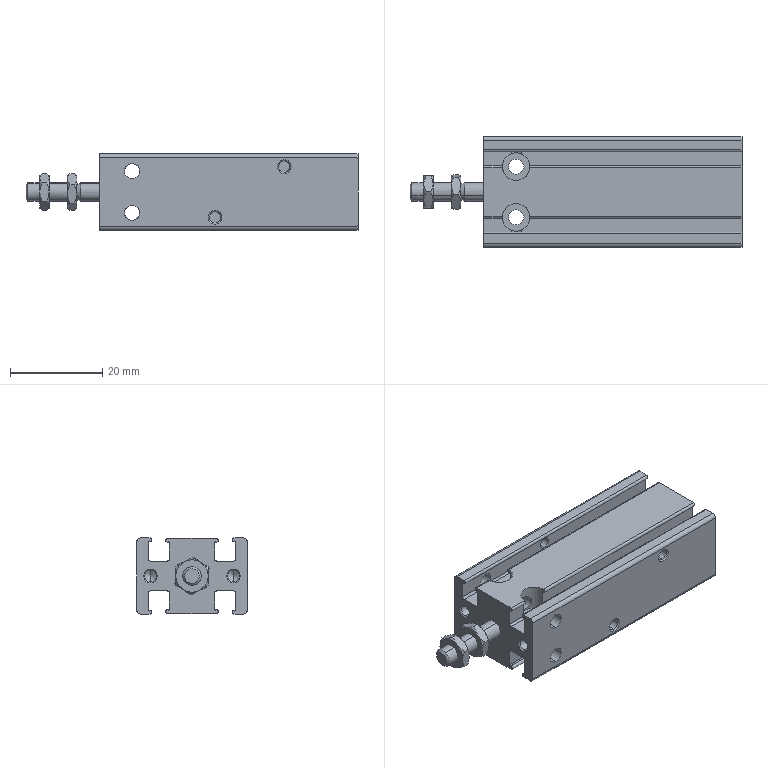Part | SolidWorks | features CompositeCurve 1 | 4 solids | 250 faces | box 72 x 24 x 16.5 mm | volume 14994 mm3 | cylinder 127 | cone 64 | plane 59 | commonest cylinder face diameters 0.8 x35 0.4 x18 2.459 x16 3.3 x16 6 x16 4 x6